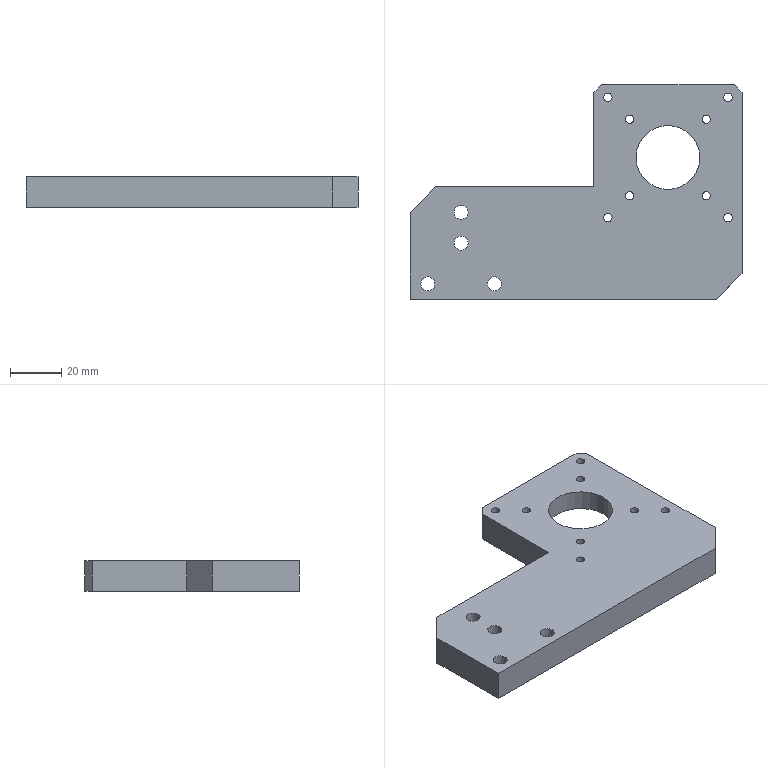Part | SolidWorks | features ICE 8, Chamfer 3, HoleWzd 3, Cut 2, Extrusion 1 | 1 solid | 56 faces | box 130 x 84 x 12 mm | volume 83062 mm3 | cylinder 39 | plane 17 | commonest cylinder face diameters 3.3 x16 5.5 x8 10 x8 40 x5 25 x2